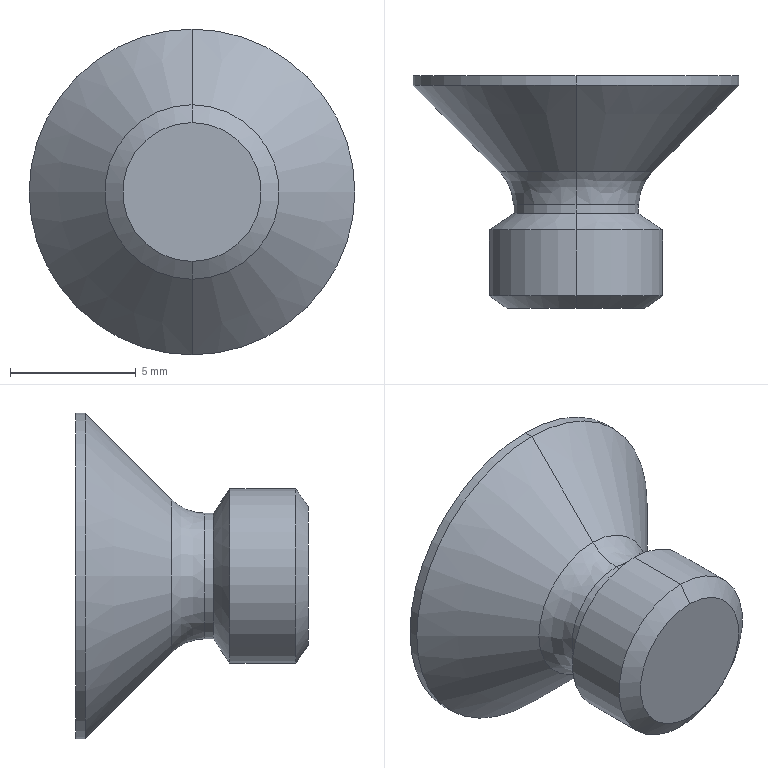Part | SolidWorks | features BaseBody 1 | 1 solid | 31 faces | box 12.923 x 9.231 x 12.923 mm | volume 413.221 mm3 | plane 17 | cylinder 6 | cone 6 | spline 2 | commonest cylinder face diameters 4.988 x2 6.923 x2 12.923 x2
STEP:
#1=CARTESIAN_POINT('',(-17.753,381.039,168.119));
#2=VERTEX_POINT('',#1);
#3=CARTESIAN_POINT('',(-17.753,381.039,174.188));
#4=VERTEX_POINT('',#3);
#5=CARTESIAN_POINT('',(-17.753,381.039,171.154));
#6=DIRECTION('',(0.,1.,0.));
#7=DIRECTION('',(1.,0.,0.));
#8=AXIS2_PLACEMENT_3D('',#5,#6,#7);
#9=CIRCLE('',#8,3.035);
#10=EDGE_CURVE('',#2,#4,#9,.T.);
#11=ORIENTED_EDGE('',*,*,#10,.F.);
#12=CARTESIAN_POINT('',(-17.753,379.733,168.66));
#13=VERTEX_POINT('',#12);
#14=CARTESIAN_POINT('',(-17.753,379.733,166.814));
#15=DIRECTION('',(1.,0.,0.));
#16=DIRECTION('',(0.,0.,-1.));
#17=AXIS2_PLACEMENT_3D('',#14,#15,#16);
#18=CIRCLE('',#17,1.846);
#19=EDGE_CURVE('',#2,#13,#18,.T.);
#20=ORIENTED_EDGE('',*,*,#19,.T.);
#21=CARTESIAN_POINT('',(-17.753,379.733,173.648));
#22=VERTEX_POINT('',#21);
#23=CARTESIAN_POINT('',(-17.753,379.733,171.154));
#24=DIRECTION('',(0.,-1.,0.));
#25=DIRECTION('',(0.,0.,1.));
#26=AXIS2_PLACEMENT_3D('',#23,#24,#25);
#27=CIRCLE('',#26,2.494);
#28=EDGE_CURVE('',#22,#13,#27,.T.);
#29=ORIENTED_EDGE('',*,*,#28,.F.);
#30=CARTESIAN_POINT('',(-17.753,379.733,175.494));
#31=DIRECTION('',(-1.,0.,0.));
#32=DIRECTION('',(0.,0.,1.));
#33=AXIS2_PLACEMENT_3D('',#30,#31,#32);
#34=CIRCLE('',#33,1.846);
#35=EDGE_CURVE('',#4,#22,#34,.T.);
#36=ORIENTED_EDGE('',*,*,#35,.F.);
#37=EDGE_LOOP('',(#11,#20,#29,#36));
#38=FACE_OUTER_BOUND('',#37,.T.);
#39=CARTESIAN_POINT('',(-17.753,381.039,174.188));
#40=CARTESIAN_POINT('',(-23.823,381.039,174.188));
#41=CARTESIAN_POINT('',(-23.823,381.039,168.119));
#42=CARTESIAN_POINT('',(-17.753,381.039,168.119));
#43=CARTESIAN_POINT('',(-17.753,380.688,173.838));
#44=CARTESIAN_POINT('',(-23.121,380.688,173.838));
#45=CARTESIAN_POINT('',(-23.121,380.688,168.47));
#46=CARTESIAN_POINT('',(-17.753,380.688,168.47));
#47=CARTESIAN_POINT('',(-17.753,380.229,173.648));
#48=CARTESIAN_POINT('',(-22.741,380.229,173.648));
#49=CARTESIAN_POINT('',(-22.741,380.229,168.66));
#50=CARTESIAN_POINT('',(-17.753,380.229,168.66));
#51=CARTESIAN_POINT('',(-17.753,379.733,173.648));
#52=CARTESIAN_POINT('',(-22.741,379.733,173.648));
#53=CARTESIAN_POINT('',(-22.741,379.733,168.66));
#54=CARTESIAN_POINT('',(-17.753,379.733,168.66));
#55=(BOUNDED_SURFACE()B_SPLINE_SURFACE(3,3,((#39,#40,#41,#42),(#43,#44,#45,#46),(#47,#48,#49,#50),(#51,#52,#53,#54)),.UNSPECIFIED.,.F.,.F.,.F.)B_SPLINE_SURFACE_WITH_KNOTS((4,4),(4,4),(0.,1.),(0.,1.),.UNSPECIFIED.)GEOMETRIC_REPRESENTATION_ITEM()RATIONAL_B_SPLINE_SURFACE(((1.,0.3333,0.3333,1.),(0.9493,0.3164,0.3164,0.9493),(0.9493,0.3164,0.3164,0.9493),(1.,0.3333,0.3333,1.)))REPRESENTATION_ITEM('')SURFACE());
#56=ADVANCED_FACE('',(#38),#55,.F.);
#57=CARTESIAN_POINT('',(-17.753,384.465,177.615));
#58=VERTEX_POINT('',#57);
#59=CARTESIAN_POINT('',(-17.753,384.465,164.692));
#60=VERTEX_POINT('',#59);
#61=CARTESIAN_POINT('',(-17.753,384.465,171.154));
#62=DIRECTION('',(0.,1.,0.));
#63=DIRECTION('',(0.,0.,1.));
#64=AXIS2_PLACEMENT_3D('',#61,#62,#63);
#65=CIRCLE('',#64,6.462);
#66=EDGE_CURVE('',#58,#60,#65,.T.);
#67=ORIENTED_EDGE('',*,*,#66,.T.);
#68=CARTESIAN_POINT('',(-17.753,384.846,164.692));
#69=VERTEX_POINT('',#68);
#70=CARTESIAN_POINT('',(-17.753,375.615,164.692));
#71=DIRECTION('',(0.,1.,0.));
#72=VECTOR('',#71,1000.);
#73=LINE('',#70,#72);
#74=EDGE_CURVE('',#60,#69,#73,.T.);
#75=ORIENTED_EDGE('',*,*,#74,.T.);
#76=CARTESIAN_POINT('',(-17.753,384.846,177.615));
#77=VERTEX_POINT('',#76);
#78=CARTESIAN_POINT('',(-17.753,384.846,171.154));
#79=DIRECTION('',(0.,-1.,0.));
#80=DIRECTION('',(0.,0.,1.));
#81=AXIS2_PLACEMENT_3D('',#78,#79,#80);
#82=CIRCLE('',#81,6.462);
#83=EDGE_CURVE('',#69,#77,#82,.T.);
#84=ORIENTED_EDGE('',*,*,#83,.T.);
#85=CARTESIAN_POINT('',(-17.753,375.615,177.615));
#86=DIRECTION('',(0.,1.,0.));
#87=VECTOR('',#86,1000.);
#88=LINE('',#85,#87);
#89=EDGE_CURVE('',#58,#77,#88,.T.);
#90=ORIENTED_EDGE('',*,*,#89,.F.);
#91=EDGE_LOOP('',(#67,#75,#84,#90));
#92=FACE_OUTER_BOUND('',#91,.T.);
#93=CARTESIAN_POINT('',(-17.753,375.615,171.154));
#94=DIRECTION('',(0.,1.,0.));
#95=DIRECTION('',(0.,0.,1.));
#96=AXIS2_PLACEMENT_3D('',#93,#94,#95);
#97=CYLINDRICAL_SURFACE('',#96,6.462);
#98=ADVANCED_FACE('',(#92),#97,.T.);
#99=CARTESIAN_POINT('',(-17.753,381.039,171.154));
#100=DIRECTION('',(0.,1.,0.));
#101=DIRECTION('',(1.,0.,0.));
#102=AXIS2_PLACEMENT_3D('',#99,#100,#101);
#103=CIRCLE('',#102,3.035);
#104=EDGE_CURVE('',#4,#2,#103,.T.);
#105=ORIENTED_EDGE('',*,*,#104,.T.);
#106=CARTESIAN_POINT('',(-17.753,384.465,164.692));
#107=DIRECTION('',(0.,0.7071,-0.7071));
#108=VECTOR('',#107,1000.);
#109=LINE('',#106,#108);
#110=EDGE_CURVE('',#2,#60,#109,.T.);
#111=ORIENTED_EDGE('',*,*,#110,.T.);
#112=ORIENTED_EDGE('',*,*,#66,.F.);
#113=CARTESIAN_POINT('',(-17.753,384.465,177.615));
#114=DIRECTION('',(0.,0.7071,0.7071));
#115=VECTOR('',#114,1000.);
#116=LINE('',#113,#115);
#117=EDGE_CURVE('',#4,#58,#116,.T.);
#118=ORIENTED_EDGE('',*,*,#117,.F.);
#119=EDGE_LOOP('',(#105,#111,#112,#118));
#120=FACE_OUTER_BOUND('',#119,.T.);
#121=CARTESIAN_POINT('',(-17.753,384.465,171.154));
#122=DIRECTION('',(0.,1.,0.));
#123=DIRECTION('',(0.,0.,1.));
#124=AXIS2_PLACEMENT_3D('',#121,#122,#123);
#125=CONICAL_SURFACE('',#124,6.462,0.7854);
#126=ADVANCED_FACE('',(#120),#125,.T.);
#127=CARTESIAN_POINT('',(-17.753,379.38,173.648));
#128=VERTEX_POINT('',#127);
#129=CARTESIAN_POINT('',(-17.753,379.38,168.66));
#130=VERTEX_POINT('',#129);
#131=CARTESIAN_POINT('',(-17.753,379.38,171.154));
#132=DIRECTION('',(0.,1.,0.));
#133=DIRECTION('',(0.,0.,1.));
#134=AXIS2_PLACEMENT_3D('',#131,#132,#133);
#135=CIRCLE('',#134,2.494);
#136=EDGE_CURVE('',#128,#130,#135,.T.);
#137=ORIENTED_EDGE('',*,*,#136,.T.);
#138=CARTESIAN_POINT('',(-17.753,375.615,168.66));
#139=DIRECTION('',(0.,1.,0.));
#140=VECTOR('',#139,1000.);
#141=LINE('',#138,#140);
#142=EDGE_CURVE('',#130,#13,#141,.T.);
#143=ORIENTED_EDGE('',*,*,#142,.T.);
#144=CARTESIAN_POINT('',(-17.753,379.733,171.154));
#145=DIRECTION('',(0.,-1.,0.));
#146=DIRECTION('',(0.,0.,1.));
#147=AXIS2_PLACEMENT_3D('',#144,#145,#146);
#148=CIRCLE('',#147,2.494);
#149=EDGE_CURVE('',#13,#22,#148,.T.);
#150=ORIENTED_EDGE('',*,*,#149,.T.);
#151=CARTESIAN_POINT('',(-17.753,375.615,173.648));
#152=DIRECTION('',(0.,1.,0.));
#153=VECTOR('',#152,1000.);
#154=LINE('',#151,#153);
#155=EDGE_CURVE('',#128,#22,#154,.T.);
#156=ORIENTED_EDGE('',*,*,#155,.F.);
#157=EDGE_LOOP('',(#137,#143,#150,#156));
#158=FACE_OUTER_BOUND('',#157,.T.);
#159=CARTESIAN_POINT('',(-17.753,375.615,171.154));
#160=DIRECTION('',(0.,1.,0.));
#161=DIRECTION('',(0.,0.,1.));
#162=AXIS2_PLACEMENT_3D('',#159,#160,#161);
#163=CYLINDRICAL_SURFACE('',#162,2.494);
#164=ADVANCED_FACE('',(#158),#163,.T.);
#165=ORIENTED_EDGE('',*,*,#136,.F.);
#166=CARTESIAN_POINT('',(-17.753,378.731,174.615));
#167=VERTEX_POINT('',#166);
#168=CARTESIAN_POINT('',(-17.753,378.731,174.615));
#169=DIRECTION('',(0.,-0.5573,0.8303));
#170=VECTOR('',#169,1000.);
#171=LINE('',#168,#170);
#172=EDGE_CURVE('',#128,#167,#171,.T.);
#173=ORIENTED_EDGE('',*,*,#172,.T.);
#174=CARTESIAN_POINT('',(-17.753,378.731,167.692));
#175=VERTEX_POINT('',#174);
#176=CARTESIAN_POINT('',(-17.753,378.731,171.154));
#177=DIRECTION('',(0.,1.,0.));
#178=DIRECTION('',(0.,0.,-1.));
#179=AXIS2_PLACEMENT_3D('',#176,#177,#178);
#180=CIRCLE('',#179,3.462);
#181=EDGE_CURVE('',#167,#175,#180,.T.);
#182=ORIENTED_EDGE('',*,*,#181,.T.);
#183=CARTESIAN_POINT('',(-17.753,378.731,167.692));
#184=DIRECTION('',(0.,-0.5573,-0.8303));
#185=VECTOR('',#184,1000.);
#186=LINE('',#183,#185);
#187=EDGE_CURVE('',#130,#175,#186,.T.);
#188=ORIENTED_EDGE('',*,*,#187,.F.);
#189=EDGE_LOOP('',(#165,#173,#182,#188));
#190=FACE_OUTER_BOUND('',#189,.T.);
#191=CARTESIAN_POINT('',(-17.753,378.731,171.154));
#192=DIRECTION('',(0.,-1.,0.));
#193=DIRECTION('',(0.,0.,-1.));
#194=AXIS2_PLACEMENT_3D('',#191,#192,#193);
#195=CONICAL_SURFACE('',#194,3.462,0.9796);
#196=ADVANCED_FACE('',(#190),#195,.T.);
#197=CARTESIAN_POINT('',(-17.753,376.116,174.615));
#198=VERTEX_POINT('',#197);
#199=CARTESIAN_POINT('',(-17.753,376.116,167.692));
#200=VERTEX_POINT('',#199);
#201=CARTESIAN_POINT('',(-17.753,376.116,171.154));
#202=DIRECTION('',(0.,1.,0.));
#203=DIRECTION('',(0.,0.,1.));
#204=AXIS2_PLACEMENT_3D('',#201,#202,#203);
#205=CIRCLE('',#204,3.462);
#206=EDGE_CURVE('',#198,#200,#205,.T.);
#207=ORIENTED_EDGE('',*,*,#206,.T.);
#208=CARTESIAN_POINT('',(-17.753,375.615,167.692));
#209=DIRECTION('',(0.,1.,0.));
#210=VECTOR('',#209,1000.);
#211=LINE('',#208,#210);
#212=EDGE_CURVE('',#200,#175,#211,.T.);
#213=ORIENTED_EDGE('',*,*,#212,.T.);
#214=ORIENTED_EDGE('',*,*,#181,.F.);
#215=CARTESIAN_POINT('',(-17.753,375.615,174.615));
#216=DIRECTION('',(0.,1.,0.));
#217=VECTOR('',#216,1000.);
#218=LINE('',#215,#217);
#219=EDGE_CURVE('',#198,#167,#218,.T.);
#220=ORIENTED_EDGE('',*,*,#219,.F.);
#221=EDGE_LOOP('',(#207,#213,#214,#220));
#222=FACE_OUTER_BOUND('',#221,.T.);
#223=CARTESIAN_POINT('',(-17.753,375.615,171.154));
#224=DIRECTION('',(0.,1.,0.));
#225=DIRECTION('',(0.,0.,1.));
#226=AXIS2_PLACEMENT_3D('',#223,#224,#225);
#227=CYLINDRICAL_SURFACE('',#226,3.462);
#228=ADVANCED_FACE('',(#222),#227,.T.);
#229=CARTESIAN_POINT('',(-17.753,375.615,173.908));
#230=VERTEX_POINT('',#229);
#231=CARTESIAN_POINT('',(-17.753,375.615,168.4));
#232=VERTEX_POINT('',#231);
#233=CARTESIAN_POINT('',(-17.753,375.615,171.154));
#234=DIRECTION('',(0.,1.,0.));
#235=DIRECTION('',(0.,0.,1.));
#236=AXIS2_PLACEMENT_3D('',#233,#234,#235);
#237=CIRCLE('',#236,2.754);
#238=EDGE_CURVE('',#230,#232,#237,.T.);
#239=ORIENTED_EDGE('',*,*,#238,.T.);
#240=CARTESIAN_POINT('',(-17.753,376.116,167.692));
#241=DIRECTION('',(0.,0.5774,-0.8165));
#242=VECTOR('',#241,1000.);
#243=LINE('',#240,#242);
#244=EDGE_CURVE('',#232,#200,#243,.T.);
#245=ORIENTED_EDGE('',*,*,#244,.T.);
#246=ORIENTED_EDGE('',*,*,#206,.F.);
#247=CARTESIAN_POINT('',(-17.753,376.116,174.615));
#248=DIRECTION('',(0.,0.5774,0.8165));
#249=VECTOR('',#248,1000.);
#250=LINE('',#247,#249);
#251=EDGE_CURVE('',#230,#198,#250,.T.);
#252=ORIENTED_EDGE('',*,*,#251,.F.);
#253=EDGE_LOOP('',(#239,#245,#246,#252));
#254=FACE_OUTER_BOUND('',#253,.T.);
#255=CARTESIAN_POINT('',(-17.753,376.116,171.154));
#256=DIRECTION('',(0.,1.,0.));
#257=DIRECTION('',(0.,0.,1.));
#258=AXIS2_PLACEMENT_3D('',#255,#256,#257);
#259=CONICAL_SURFACE('',#258,3.462,0.9553);
#260=ADVANCED_FACE('',(#254),#259,.T.);
#261=CARTESIAN_POINT('',(-21.1,384.846,170.317));
#262=VERTEX_POINT('',#261);
#263=CARTESIAN_POINT('',(-21.1,384.846,171.99));
#264=VERTEX_POINT('',#263);
#265=CARTESIAN_POINT('',(-21.1,384.846,171.154));
#266=DIRECTION('',(0.,0.,1.));
#267=VECTOR('',#266,1000.);
#268=LINE('',#265,#267);
#269=EDGE_CURVE('',#262,#264,#268,.T.);
#270=ORIENTED_EDGE('',*,*,#269,.F.);
#271=CARTESIAN_POINT('',(-18.59,384.846,170.317));
#272=VERTEX_POINT('',#271);
#273=CARTESIAN_POINT('',(-17.753,384.846,170.317));
#274=DIRECTION('',(-1.,0.,0.));
#275=VECTOR('',#274,1000.);
#276=LINE('',#273,#275);
#277=EDGE_CURVE('',#272,#262,#276,.T.);
#278=ORIENTED_EDGE('',*,*,#277,.F.);
#279=CARTESIAN_POINT('',(-18.59,384.846,167.808));
#280=VERTEX_POINT('',#279);
#281=CARTESIAN_POINT('',(-18.59,384.846,171.154));
#282=DIRECTION('',(0.,0.,1.));
#283=VECTOR('',#282,1000.);
#284=LINE('',#281,#283);
#285=EDGE_CURVE('',#280,#272,#284,.T.);
#286=ORIENTED_EDGE('',*,*,#285,.F.);
#287=CARTESIAN_POINT('',(-16.917,384.846,167.808));
#288=VERTEX_POINT('',#287);
#289=CARTESIAN_POINT('',(-17.753,384.846,167.808));
#290=DIRECTION('',(-1.,0.,0.));
#291=VECTOR('',#290,1000.);
#292=LINE('',#289,#291);
#293=EDGE_CURVE('',#288,#280,#292,.T.);
#294=ORIENTED_EDGE('',*,*,#293,.F.);
#295=CARTESIAN_POINT('',(-16.917,384.846,170.317));
#296=VERTEX_POINT('',#295);
#297=CARTESIAN_POINT('',(-16.917,384.846,171.154));
#298=DIRECTION('',(0.,0.,-1.));
#299=VECTOR('',#298,1000.);
#300=LINE('',#297,#299);
#301=EDGE_CURVE('',#296,#288,#300,.T.);
#302=ORIENTED_EDGE('',*,*,#301,.F.);
#303=CARTESIAN_POINT('',(-14.407,384.846,170.317));
#304=VERTEX_POINT('',#303);
#305=CARTESIAN_POINT('',(-17.753,384.846,170.317));
#306=DIRECTION('',(-1.,0.,0.));
#307=VECTOR('',#306,1000.);
#308=LINE('',#305,#307);
#309=EDGE_CURVE('',#304,#296,#308,.T.);
#310=ORIENTED_EDGE('',*,*,#309,.F.);
#311=CARTESIAN_POINT('',(-14.407,384.846,171.99));
#312=VERTEX_POINT('',#311);
#313=CARTESIAN_POINT('',(-14.407,384.846,171.154));
#314=DIRECTION('',(0.,0.,-1.));
#315=VECTOR('',#314,1000.);
#316=LINE('',#313,#315);
#317=EDGE_CURVE('',#312,#304,#316,.T.);
#318=ORIENTED_EDGE('',*,*,#317,.F.);
#319=CARTESIAN_POINT('',(-16.917,384.846,171.99));
#320=VERTEX_POINT('',#319);
#321=CARTESIAN_POINT('',(-17.753,384.846,171.99));
#322=DIRECTION('',(1.,0.,0.));
#323=VECTOR('',#322,1000.);
#324=LINE('',#321,#323);
#325=EDGE_CURVE('',#320,#312,#324,.T.);
#326=ORIENTED_EDGE('',*,*,#325,.F.);
#327=CARTESIAN_POINT('',(-16.917,384.846,174.5));
#328=VERTEX_POINT('',#327);
#329=CARTESIAN_POINT('',(-16.917,384.846,171.154));
#330=DIRECTION('',(0.,0.,-1.));
#331=VECTOR('',#330,1000.);
#332=LINE('',#329,#331);
#333=EDGE_CURVE('',#328,#320,#332,.T.);
#334=ORIENTED_EDGE('',*,*,#333,.F.);
#335=CARTESIAN_POINT('',(-18.59,384.846,174.5));
#336=VERTEX_POINT('',#335);
#337=CARTESIAN_POINT('',(-17.753,384.846,174.5));
#338=DIRECTION('',(1.,0.,0.));
#339=VECTOR('',#338,1000.);
#340=LINE('',#337,#339);
#341=EDGE_CURVE('',#336,#328,#340,.T.);
#342=ORIENTED_EDGE('',*,*,#341,.F.);
#343=CARTESIAN_POINT('',(-18.59,384.846,171.99));
#344=VERTEX_POINT('',#343);
#345=CARTESIAN_POINT('',(-18.59,384.846,171.154));
#346=DIRECTION('',(0.,0.,1.));
#347=VECTOR('',#346,1000.);
#348=LINE('',#345,#347);
#349=EDGE_CURVE('',#344,#336,#348,.T.);
#350=ORIENTED_EDGE('',*,*,#349,.F.);
#351=CARTESIAN_POINT('',(-17.753,384.846,171.99));
#352=DIRECTION('',(1.,0.,0.));
#353=VECTOR('',#352,1000.);
#354=LINE('',#351,#353);
#355=EDGE_CURVE('',#264,#344,#354,.T.);
#356=ORIENTED_EDGE('',*,*,#355,.F.);
#357=EDGE_LOOP('',(#270,#278,#286,#294,#302,#310,#318,#326,#334,#342,#350,#356));
#358=FACE_BOUND('',#357,.T.);
#359=CARTESIAN_POINT('',(-17.753,384.846,171.154));
#360=DIRECTION('',(0.,-1.,0.));
#361=DIRECTION('',(0.,0.,1.));
#362=AXIS2_PLACEMENT_3D('',#359,#360,#361);
#363=CIRCLE('',#362,6.462);
#364=EDGE_CURVE('',#77,#69,#363,.T.);
#365=ORIENTED_EDGE('',*,*,#364,.F.);
#366=ORIENTED_EDGE('',*,*,#83,.F.);
#367=EDGE_LOOP('',(#365,#366));
#368=FACE_OUTER_BOUND('',#367,.T.);
#369=CARTESIAN_POINT('',(-17.753,384.846,171.154));
#370=DIRECTION('',(0.,-1.,0.));
#371=DIRECTION('',(0.,0.,-1.));
#372=AXIS2_PLACEMENT_3D('',#369,#370,#371);
#373=PLANE('',#372);
#374=ADVANCED_FACE('',(#358,#368),#373,.F.);
#375=CARTESIAN_POINT('',(-21.1,382.942,171.99));
#376=VERTEX_POINT('',#375);
#377=CARTESIAN_POINT('',(-21.1,384.846,171.99));
#378=DIRECTION('',(0.,-1.,0.));
#379=VECTOR('',#378,1000.);
#380=LINE('',#377,#379);
#381=EDGE_CURVE('',#264,#376,#380,.T.);
#382=ORIENTED_EDGE('',*,*,#381,.F.);
#383=ORIENTED_EDGE('',*,*,#355,.T.);
#384=CARTESIAN_POINT('',(-18.59,381.241,171.99));
#385=VERTEX_POINT('',#384);
#386=CARTESIAN_POINT('',(-18.59,384.846,171.99));
#387=DIRECTION('',(0.,1.,0.));
#388=VECTOR('',#387,1000.);
#389=LINE('',#386,#388);
#390=EDGE_CURVE('',#385,#344,#389,.T.);
#391=ORIENTED_EDGE('',*,*,#390,.F.);
#392=CARTESIAN_POINT('',(-21.1,382.942,171.99));
#393=DIRECTION('',(0.8278,-0.5611,0.));
#394=VECTOR('',#393,1000.);
#395=LINE('',#392,#394);
#396=EDGE_CURVE('',#376,#385,#395,.T.);
#397=ORIENTED_EDGE('',*,*,#396,.F.);
#398=EDGE_LOOP('',(#382,#383,#391,#397));
#399=FACE_OUTER_BOUND('',#398,.T.);
#400=CARTESIAN_POINT('',(-17.753,384.846,171.99));
#401=DIRECTION('',(0.,0.,1.));
#402=DIRECTION('',(1.,0.,0.));
#403=AXIS2_PLACEMENT_3D('',#400,#401,#402);
#404=PLANE('',#403);
#405=ADVANCED_FACE('',(#399),#404,.F.);
#406=ORIENTED_EDGE('',*,*,#381,.T.);
#407=CARTESIAN_POINT('',(-21.1,382.942,170.317));
#408=VERTEX_POINT('',#407);
#409=CARTESIAN_POINT('',(-21.1,382.942,171.99));
#410=DIRECTION('',(0.,0.,-1.));
#411=VECTOR('',#410,1000.);
#412=LINE('',#409,#411);
#413=EDGE_CURVE('',#376,#408,#412,.T.);
#414=ORIENTED_EDGE('',*,*,#413,.T.);
#415=CARTESIAN_POINT('',(-21.1,394.458,170.317));
#416=DIRECTION('',(0.,1.,0.));
#417=VECTOR('',#416,1000.);
#418=LINE('',#415,#417);
#419=EDGE_CURVE('',#408,#262,#418,.T.);
#420=ORIENTED_EDGE('',*,*,#419,.T.);
#421=ORIENTED_EDGE('',*,*,#269,.T.);
#422=EDGE_LOOP('',(#406,#414,#420,#421));
#423=FACE_OUTER_BOUND('',#422,.T.);
#424=CARTESIAN_POINT('',(-21.1,394.458,171.99));
#425=DIRECTION('',(1.,0.,0.));
#426=DIRECTION('',(0.,0.,-1.));
#427=AXIS2_PLACEMENT_3D('',#424,#425,#426);
#428=PLANE('',#427);
#429=ADVANCED_FACE('',(#423),#428,.T.);
#430=ORIENTED_EDGE('',*,*,#277,.T.);
#431=ORIENTED_EDGE('',*,*,#419,.F.);
#432=CARTESIAN_POINT('',(-18.59,381.241,170.317));
#433=VERTEX_POINT('',#432);
#434=CARTESIAN_POINT('',(-21.1,382.942,170.317));
#435=DIRECTION('',(0.8278,-0.5611,0.));
#436=VECTOR('',#435,1000.);
#437=LINE('',#434,#436);
#438=EDGE_CURVE('',#408,#433,#437,.T.);
#439=ORIENTED_EDGE('',*,*,#438,.T.);
#440=CARTESIAN_POINT('',(-18.59,384.846,170.317));
#441=DIRECTION('',(0.,1.,0.));
#442=VECTOR('',#441,1000.);
#443=LINE('',#440,#442);
#444=EDGE_CURVE('',#433,#272,#443,.T.);
#445=ORIENTED_EDGE('',*,*,#444,.T.);
#446=EDGE_LOOP('',(#430,#431,#439,#445));
#447=FACE_OUTER_BOUND('',#446,.T.);
#448=CARTESIAN_POINT('',(-17.753,384.846,170.317));
#449=DIRECTION('',(0.,0.,1.));
#450=DIRECTION('',(1.,0.,0.));
#451=AXIS2_PLACEMENT_3D('',#448,#449,#450);
#452=PLANE('',#451);
#453=ADVANCED_FACE('',(#447),#452,.T.);
#454=CARTESIAN_POINT('',(-18.59,382.942,167.808));
#455=VERTEX_POINT('',#454);
#456=CARTESIAN_POINT('',(-18.59,381.01,170.317));
#457=VERTEX_POINT('',#456);
#458=CARTESIAN_POINT('',(-18.59,382.942,167.808));
#459=DIRECTION('',(0.,-0.61,0.7924));
#460=VECTOR('',#459,1000.);
#461=LINE('',#458,#460);
#462=EDGE_CURVE('',#455,#457,#461,.T.);
#463=ORIENTED_EDGE('',*,*,#462,.F.);
#464=CARTESIAN_POINT('',(-18.59,384.846,167.808));
#465=DIRECTION('',(0.,-1.,0.));
#466=VECTOR('',#465,1000.);
#467=LINE('',#464,#466);
#468=EDGE_CURVE('',#280,#455,#467,.T.);
#469=ORIENTED_EDGE('',*,*,#468,.F.);
#470=ORIENTED_EDGE('',*,*,#285,.T.);
#471=ORIENTED_EDGE('',*,*,#444,.F.);
#472=CARTESIAN_POINT('',(-18.59,381.241,171.154));
#473=DIRECTION('',(0.,0.,-1.));
#474=VECTOR('',#473,1000.);
#475=LINE('',#472,#474);
#476=EDGE_CURVE('',#385,#433,#475,.T.);
#477=ORIENTED_EDGE('',*,*,#476,.F.);
#478=ORIENTED_EDGE('',*,*,#390,.T.);
#479=ORIENTED_EDGE('',*,*,#349,.T.);
#480=CARTESIAN_POINT('',(-18.59,382.942,174.5));
#481=VERTEX_POINT('',#480);
#482=CARTESIAN_POINT('',(-18.59,384.846,174.5));
#483=DIRECTION('',(0.,1.,0.));
#484=VECTOR('',#483,1000.);
#485=LINE('',#482,#484);
#486=EDGE_CURVE('',#481,#336,#485,.T.);
#487=ORIENTED_EDGE('',*,*,#486,.F.);
#488=CARTESIAN_POINT('',(-18.59,381.01,171.99));
#489=VERTEX_POINT('',#488);
#490=CARTESIAN_POINT('',(-18.59,381.01,171.99));
#491=DIRECTION('',(0.,0.61,0.7924));
#492=VECTOR('',#491,1000.);
#493=LINE('',#490,#492);
#494=EDGE_CURVE('',#489,#481,#493,.T.);
#495=ORIENTED_EDGE('',*,*,#494,.F.);
#496=CARTESIAN_POINT('',(-18.59,381.01,171.154));
#497=DIRECTION('',(0.,0.,1.));
#498=VECTOR('',#497,1000.);
#499=LINE('',#496,#498);
#500=EDGE_CURVE('',#457,#489,#499,.T.);
#501=ORIENTED_EDGE('',*,*,#500,.F.);
#502=EDGE_LOOP('',(#463,#469,#470,#471,#477,#478,#479,#487,#495,#501));
#503=FACE_OUTER_BOUND('',#502,.T.);
#504=CARTESIAN_POINT('',(-18.59,384.846,171.154));
#505=DIRECTION('',(-1.,0.,0.));
#506=DIRECTION('',(0.,0.,1.));
#507=AXIS2_PLACEMENT_3D('',#504,#505,#506);
#508=PLANE('',#507);
#509=ADVANCED_FACE('',(#503),#508,.F.);
#510=ORIENTED_EDGE('',*,*,#468,.T.);
#511=CARTESIAN_POINT('',(-16.917,382.942,167.808));
#512=VERTEX_POINT('',#511);
#513=CARTESIAN_POINT('',(-18.59,382.942,167.808));
#514=DIRECTION('',(1.,0.,0.));
#515=VECTOR('',#514,1000.);
#516=LINE('',#513,#515);
#517=EDGE_CURVE('',#455,#512,#516,.T.);
#518=ORIENTED_EDGE('',*,*,#517,.T.);
#519=CARTESIAN_POINT('',(-16.917,385.227,167.808));
#520=DIRECTION('',(0.,1.,0.));
#521=VECTOR('',#520,1000.);
#522=LINE('',#519,#521);
#523=EDGE_CURVE('',#512,#288,#522,.T.);
#524=ORIENTED_EDGE('',*,*,#523,.T.);
#525=ORIENTED_EDGE('',*,*,#293,.T.);
#526=EDGE_LOOP('',(#510,#518,#524,#525));
#527=FACE_OUTER_BOUND('',#526,.T.);
#528=CARTESIAN_POINT('',(-18.59,385.227,167.808));
#529=DIRECTION('',(0.,0.,1.));
#530=DIRECTION('',(1.,0.,0.));
#531=AXIS2_PLACEMENT_3D('',#528,#529,#530);
#532=PLANE('',#531);
#533=ADVANCED_FACE('',(#527),#532,.T.);
#534=CARTESIAN_POINT('',(-16.917,381.01,170.317));
#535=VERTEX_POINT('',#534);
#536=CARTESIAN_POINT('',(-16.917,381.01,171.99));
#537=VERTEX_POINT('',#536);
#538=CARTESIAN_POINT('',(-16.917,381.01,171.154));
#539=DIRECTION('',(0.,0.,1.));
#540=VECTOR('',#539,1000.);
#541=LINE('',#538,#540);
#542=EDGE_CURVE('',#535,#537,#541,.T.);
#543=ORIENTED_EDGE('',*,*,#542,.T.);
#544=CARTESIAN_POINT('',(-16.917,382.942,174.5));
#545=VERTEX_POINT('',#544);
#546=CARTESIAN_POINT('',(-16.917,381.01,171.99));
#547=DIRECTION('',(0.,0.61,0.7924));
#548=VECTOR('',#547,1000.);
#549=LINE('',#546,#548);
#550=EDGE_CURVE('',#537,#545,#549,.T.);
#551=ORIENTED_EDGE('',*,*,#550,.T.);
#552=CARTESIAN_POINT('',(-16.917,384.846,174.5));
#553=DIRECTION('',(0.,1.,0.));
#554=VECTOR('',#553,1000.);
#555=LINE('',#552,#554);
#556=EDGE_CURVE('',#545,#328,#555,.T.);
#557=ORIENTED_EDGE('',*,*,#556,.T.);
#558=ORIENTED_EDGE('',*,*,#333,.T.);
#559=CARTESIAN_POINT('',(-16.917,381.241,171.99));
#560=VERTEX_POINT('',#559);
#561=CARTESIAN_POINT('',(-16.917,384.846,171.99));
#562=DIRECTION('',(0.,-1.,0.));
#563=VECTOR('',#562,1000.);
#564=LINE('',#561,#563);
#565=EDGE_CURVE('',#320,#560,#564,.T.);
#566=ORIENTED_EDGE('',*,*,#565,.T.);
#567=CARTESIAN_POINT('',(-16.917,381.241,170.317));
#568=VERTEX_POINT('',#567);
#569=CARTESIAN_POINT('',(-16.917,381.241,171.154));
#570=DIRECTION('',(0.,0.,-1.));
#571=VECTOR('',#570,1000.);
#572=LINE('',#569,#571);
#573=EDGE_CURVE('',#560,#568,#572,.T.);
#574=ORIENTED_EDGE('',*,*,#573,.T.);
#575=CARTESIAN_POINT('',(-16.917,384.846,170.317));
#576=DIRECTION('',(0.,1.,0.));
#577=VECTOR('',#576,1000.);
#578=LINE('',#575,#577);
#579=EDGE_CURVE('',#568,#296,#578,.T.);
#580=ORIENTED_EDGE('',*,*,#579,.T.);
#581=ORIENTED_EDGE('',*,*,#301,.T.);
#582=ORIENTED_EDGE('',*,*,#523,.F.);
#583=CARTESIAN_POINT('',(-16.917,382.942,167.808));
#584=DIRECTION('',(0.,-0.61,0.7924));
#585=VECTOR('',#584,1000.);
#586=LINE('',#583,#585);
#587=EDGE_CURVE('',#512,#535,#586,.T.);
#588=ORIENTED_EDGE('',*,*,#587,.T.);
#589=EDGE_LOOP('',(#543,#551,#557,#558,#566,#574,#580,#581,#582,#588));
#590=FACE_OUTER_BOUND('',#589,.T.);
#591=CARTESIAN_POINT('',(-16.917,384.846,171.154));
#592=DIRECTION('',(-1.,0.,0.));
#593=DIRECTION('',(0.,0.,1.));
#594=AXIS2_PLACEMENT_3D('',#591,#592,#593);
#595=PLANE('',#594);
#596=ADVANCED_FACE('',(#590),#595,.T.);
#597=ORIENTED_EDGE('',*,*,#579,.F.);
#598=CARTESIAN_POINT('',(-14.407,382.942,170.317));
#599=VERTEX_POINT('',#598);
#600=CARTESIAN_POINT('',(-16.917,381.241,170.317));
#601=DIRECTION('',(0.8278,0.5611,0.));
#602=VECTOR('',#601,1000.);
#603=LINE('',#600,#602);
#604=EDGE_CURVE('',#568,#599,#603,.T.);
#605=ORIENTED_EDGE('',*,*,#604,.T.);
#606=CARTESIAN_POINT('',(-14.407,384.846,170.317));
#607=DIRECTION('',(0.,1.,0.));
#608=VECTOR('',#607,1000.);
#609=LINE('',#606,#608);
#610=EDGE_CURVE('',#599,#304,#609,.T.);
#611=ORIENTED_EDGE('',*,*,#610,.T.);
#612=ORIENTED_EDGE('',*,*,#309,.T.);
#613=EDGE_LOOP('',(#597,#605,#611,#612));
#614=FACE_OUTER_BOUND('',#613,.T.);
#615=CARTESIAN_POINT('',(-17.753,384.846,170.317));
#616=DIRECTION('',(0.,0.,1.));
#617=DIRECTION('',(1.,0.,0.));
#618=AXIS2_PLACEMENT_3D('',#615,#616,#617);
#619=PLANE('',#618);
#620=ADVANCED_FACE('',(#614),#619,.T.);
#621=ORIENTED_EDGE('',*,*,#317,.T.);
#622=ORIENTED_EDGE('',*,*,#610,.F.);
#623=CARTESIAN_POINT('',(-14.407,382.942,171.99));
#624=VERTEX_POINT('',#623);
#625=CARTESIAN_POINT('',(-14.407,382.942,171.99));
#626=DIRECTION('',(0.,0.,1.));
#627=VECTOR('',#626,1000.);
#628=LINE('',#625,#627);
#629=EDGE_CURVE('',#599,#624,#628,.T.);
#630=ORIENTED_EDGE('',*,*,#629,.T.);
#631=CARTESIAN_POINT('',(-14.407,382.942,171.99));
#632=DIRECTION('',(0.,1.,0.));
#633=VECTOR('',#632,1000.);
#634=LINE('',#631,#633);
#635=EDGE_CURVE('',#624,#312,#634,.T.);
#636=ORIENTED_EDGE('',*,*,#635,.T.);
#637=EDGE_LOOP('',(#621,#622,#630,#636));
#638=FACE_OUTER_BOUND('',#637,.T.);
#639=CARTESIAN_POINT('',(-14.407,382.942,171.99));
#640=DIRECTION('',(-1.,0.,0.));
#641=DIRECTION('',(0.,0.,1.));
#642=AXIS2_PLACEMENT_3D('',#639,#640,#641);
#643=PLANE('',#642);
#644=ADVANCED_FACE('',(#638),#643,.T.);
#645=CARTESIAN_POINT('',(-16.917,381.241,171.99));
#646=DIRECTION('',(0.8278,0.5611,0.));
#647=VECTOR('',#646,1000.);
#648=LINE('',#645,#647);
#649=EDGE_CURVE('',#560,#624,#648,.T.);
#650=ORIENTED_EDGE('',*,*,#649,.F.);
#651=ORIENTED_EDGE('',*,*,#565,.F.);
#652=ORIENTED_EDGE('',*,*,#325,.T.);
#653=ORIENTED_EDGE('',*,*,#635,.F.);
#654=EDGE_LOOP('',(#650,#651,#652,#653));
#655=FACE_OUTER_BOUND('',#654,.T.);
#656=CARTESIAN_POINT('',(-17.753,384.846,171.99));
#657=DIRECTION('',(0.,0.,1.));
#658=DIRECTION('',(1.,0.,0.));
#659=AXIS2_PLACEMENT_3D('',#656,#657,#658);
#660=PLANE('',#659);
#661=ADVANCED_FACE('',(#655),#660,.F.);
#662=ORIENTED_EDGE('',*,*,#556,.F.);
#663=CARTESIAN_POINT('',(-18.59,382.942,174.5));
#664=DIRECTION('',(-1.,0.,0.));
#665=VECTOR('',#664,1000.);
#666=LINE('',#663,#665);
#667=EDGE_CURVE('',#545,#481,#666,.T.);
#668=ORIENTED_EDGE('',*,*,#667,.T.);
#669=ORIENTED_EDGE('',*,*,#486,.T.);
#670=ORIENTED_EDGE('',*,*,#341,.T.);
#671=EDGE_LOOP('',(#662,#668,#669,#670));
#672=FACE_OUTER_BOUND('',#671,.T.);
#673=CARTESIAN_POINT('',(-18.59,382.942,174.5));
#674=DIRECTION('',(0.,0.,-1.));
#675=DIRECTION('',(-1.,0.,0.));
#676=AXIS2_PLACEMENT_3D('',#673,#674,#675);
#677=PLANE('',#676);
#678=ADVANCED_FACE('',(#672),#677,.T.);
#679=ORIENTED_EDGE('',*,*,#74,.F.);
#680=CARTESIAN_POINT('',(-17.753,384.465,171.154));
#681=DIRECTION('',(0.,1.,0.));
#682=DIRECTION('',(0.,0.,1.));
#683=AXIS2_PLACEMENT_3D('',#680,#681,#682);
#684=CIRCLE('',#683,6.462);
#685=EDGE_CURVE('',#60,#58,#684,.T.);
#686=ORIENTED_EDGE('',*,*,#685,.T.);
#687=ORIENTED_EDGE('',*,*,#89,.T.);
#688=ORIENTED_EDGE('',*,*,#364,.T.);
#689=EDGE_LOOP('',(#679,#686,#687,#688));
#690=FACE_OUTER_BOUND('',#689,.T.);
#691=CARTESIAN_POINT('',(-17.753,375.615,171.154));
#692=DIRECTION('',(0.,1.,0.));
#693=DIRECTION('',(0.,0.,1.));
#694=AXIS2_PLACEMENT_3D('',#691,#692,#693);
#695=CYLINDRICAL_SURFACE('',#694,6.462);
#696=ADVANCED_FACE('',(#690),#695,.T.);
#697=ORIENTED_EDGE('',*,*,#413,.F.);
#698=ORIENTED_EDGE('',*,*,#396,.T.);
#699=ORIENTED_EDGE('',*,*,#476,.T.);
#700=ORIENTED_EDGE('',*,*,#438,.F.);
#701=EDGE_LOOP('',(#697,#698,#699,#700));
#702=FACE_OUTER_BOUND('',#701,.T.);
#703=CARTESIAN_POINT('',(-21.1,382.942,171.99));
#704=DIRECTION('',(0.5611,0.8278,0.));
#705=DIRECTION('',(-0.8278,0.5611,0.));
#706=AXIS2_PLACEMENT_3D('',#703,#704,#705);
#707=PLANE('',#706);
#708=ADVANCED_FACE('',(#702),#707,.T.);
#709=CARTESIAN_POINT('',(-18.59,381.01,170.317));
#710=DIRECTION('',(-1.,0.,0.));
#711=VECTOR('',#710,1000.);
#712=LINE('',#709,#711);
#713=EDGE_CURVE('',#535,#457,#712,.T.);
#714=ORIENTED_EDGE('',*,*,#713,.T.);
#715=ORIENTED_EDGE('',*,*,#500,.T.);
#716=CARTESIAN_POINT('',(-18.59,381.01,171.99));
#717=DIRECTION('',(1.,0.,0.));
#718=VECTOR('',#717,1000.);
#719=LINE('',#716,#718);
#720=EDGE_CURVE('',#489,#537,#719,.T.);
#721=ORIENTED_EDGE('',*,*,#720,.T.);
#722=ORIENTED_EDGE('',*,*,#542,.F.);
#723=EDGE_LOOP('',(#714,#715,#721,#722));
#724=FACE_OUTER_BOUND('',#723,.T.);
#725=CARTESIAN_POINT('',(-18.59,381.01,170.317));
#726=DIRECTION('',(0.,1.,0.));
#727=DIRECTION('',(0.,0.,1.));
#728=AXIS2_PLACEMENT_3D('',#725,#726,#727);
#729=PLANE('',#728);
#730=ADVANCED_FACE('',(#724),#729,.T.);
#731=ORIENTED_EDGE('',*,*,#517,.F.);
#732=ORIENTED_EDGE('',*,*,#462,.T.);
#733=ORIENTED_EDGE('',*,*,#713,.F.);
#734=ORIENTED_EDGE('',*,*,#587,.F.);
#735=EDGE_LOOP('',(#731,#732,#733,#734));
#736=FACE_OUTER_BOUND('',#735,.T.);
#737=CARTESIAN_POINT('',(-18.59,382.942,167.808));
#738=DIRECTION('',(0.,0.7924,0.61));
#739=DIRECTION('',(0.,-0.61,0.7924));
#740=AXIS2_PLACEMENT_3D('',#737,#738,#739);
#741=PLANE('',#740);
#742=ADVANCED_FACE('',(#736),#741,.T.);
#743=ORIENTED_EDGE('',*,*,#720,.F.);
#744=ORIENTED_EDGE('',*,*,#494,.T.);
#745=ORIENTED_EDGE('',*,*,#667,.F.);
#746=ORIENTED_EDGE('',*,*,#550,.F.);
#747=EDGE_LOOP('',(#743,#744,#745,#746));
#748=FACE_OUTER_BOUND('',#747,.T.);
#749=CARTESIAN_POINT('',(-18.59,381.01,171.99));
#750=DIRECTION('',(0.,0.7924,-0.61));
#751=DIRECTION('',(0.,0.61,0.7924));
#752=AXIS2_PLACEMENT_3D('',#749,#750,#751);
#753=PLANE('',#752);
#754=ADVANCED_FACE('',(#748),#753,.T.);
#755=ORIENTED_EDGE('',*,*,#573,.F.);
#756=ORIENTED_EDGE('',*,*,#649,.T.);
#757=ORIENTED_EDGE('',*,*,#629,.F.);
#758=ORIENTED_EDGE('',*,*,#604,.F.);
#759=EDGE_LOOP('',(#755,#756,#757,#758));
#760=FACE_OUTER_BOUND('',#759,.T.);
#761=CARTESIAN_POINT('',(-16.917,381.241,171.99));
#762=DIRECTION('',(-0.5611,0.8278,0.));
#763=DIRECTION('',(-0.8278,-0.5611,0.));
#764=AXIS2_PLACEMENT_3D('',#761,#762,#763);
#765=PLANE('',#764);
#766=ADVANCED_FACE('',(#760),#765,.T.);
#767=ORIENTED_EDGE('',*,*,#110,.F.);
#768=ORIENTED_EDGE('',*,*,#10,.T.);
#769=ORIENTED_EDGE('',*,*,#117,.T.);
#770=ORIENTED_EDGE('',*,*,#685,.F.);
#771=EDGE_LOOP('',(#767,#768,#769,#770));
#772=FACE_OUTER_BOUND('',#771,.T.);
#773=CARTESIAN_POINT('',(-17.753,384.465,171.154));
#774=DIRECTION('',(0.,1.,0.));
#775=DIRECTION('',(0.,0.,1.));
#776=AXIS2_PLACEMENT_3D('',#773,#774,#775);
#777=CONICAL_SURFACE('',#776,6.462,0.7854);
#778=ADVANCED_FACE('',(#772),#777,.T.);
#779=ORIENTED_EDGE('',*,*,#19,.F.);
#780=ORIENTED_EDGE('',*,*,#104,.F.);
#781=ORIENTED_EDGE('',*,*,#35,.T.);
#782=ORIENTED_EDGE('',*,*,#149,.F.);
#783=EDGE_LOOP('',(#779,#780,#781,#782));
#784=FACE_OUTER_BOUND('',#783,.T.);
#785=CARTESIAN_POINT('',(-17.753,381.039,168.119));
#786=CARTESIAN_POINT('',(-11.684,381.039,168.119));
#787=CARTESIAN_POINT('',(-11.684,381.039,174.188));
#788=CARTESIAN_POINT('',(-17.753,381.039,174.188));
#789=CARTESIAN_POINT('',(-17.753,380.688,168.47));
#790=CARTESIAN_POINT('',(-12.386,380.688,168.47));
#791=CARTESIAN_POINT('',(-12.386,380.688,173.838));
#792=CARTESIAN_POINT('',(-17.753,380.688,173.838));
#793=CARTESIAN_POINT('',(-17.753,380.229,168.66));
#794=CARTESIAN_POINT('',(-12.766,380.229,168.66));
#795=CARTESIAN_POINT('',(-12.766,380.229,173.648));
#796=CARTESIAN_POINT('',(-17.753,380.229,173.648));
#797=CARTESIAN_POINT('',(-17.753,379.733,168.66));
#798=CARTESIAN_POINT('',(-12.766,379.733,168.66));
#799=CARTESIAN_POINT('',(-12.766,379.733,173.648));
#800=CARTESIAN_POINT('',(-17.753,379.733,173.648));
#801=(BOUNDED_SURFACE()B_SPLINE_SURFACE(3,3,((#785,#786,#787,#788),(#789,#790,#791,#792),(#793,#794,#795,#796),(#797,#798,#799,#800)),.UNSPECIFIED.,.F.,.F.,.T.)B_SPLINE_SURFACE_WITH_KNOTS((4,4),(4,4),(0.,1.),(0.,1.),.UNSPECIFIED.)GEOMETRIC_REPRESENTATION_ITEM()RATIONAL_B_SPLINE_SURFACE(((1.,0.3333,0.3333,1.),(0.9493,0.3164,0.3164,0.9493),(0.9493,0.3164,0.3164,0.9493),(1.,0.3333,0.3333,1.)))REPRESENTATION_ITEM('')SURFACE());
#802=ADVANCED_FACE('',(#784),#801,.F.);
#803=ORIENTED_EDGE('',*,*,#142,.F.);
#804=CARTESIAN_POINT('',(-17.753,379.38,171.154));
#805=DIRECTION('',(0.,1.,0.));
#806=DIRECTION('',(0.,0.,1.));
#807=AXIS2_PLACEMENT_3D('',#804,#805,#806);
#808=CIRCLE('',#807,2.494);
#809=EDGE_CURVE('',#130,#128,#808,.T.);
#810=ORIENTED_EDGE('',*,*,#809,.T.);
#811=ORIENTED_EDGE('',*,*,#155,.T.);
#812=ORIENTED_EDGE('',*,*,#28,.T.);
#813=EDGE_LOOP('',(#803,#810,#811,#812));
#814=FACE_OUTER_BOUND('',#813,.T.);
#815=CARTESIAN_POINT('',(-17.753,375.615,171.154));
#816=DIRECTION('',(0.,1.,0.));
#817=DIRECTION('',(0.,0.,1.));
#818=AXIS2_PLACEMENT_3D('',#815,#816,#817);
#819=CYLINDRICAL_SURFACE('',#818,2.494);
#820=ADVANCED_FACE('',(#814),#819,.T.);
#821=ORIENTED_EDGE('',*,*,#172,.F.);
#822=ORIENTED_EDGE('',*,*,#809,.F.);
#823=ORIENTED_EDGE('',*,*,#187,.T.);
#824=CARTESIAN_POINT('',(-17.753,378.731,171.154));
#825=DIRECTION('',(0.,1.,0.));
#826=DIRECTION('',(0.,0.,-1.));
#827=AXIS2_PLACEMENT_3D('',#824,#825,#826);
#828=CIRCLE('',#827,3.462);
#829=EDGE_CURVE('',#175,#167,#828,.T.);
#830=ORIENTED_EDGE('',*,*,#829,.T.);
#831=EDGE_LOOP('',(#821,#822,#823,#830));
#832=FACE_OUTER_BOUND('',#831,.T.);
#833=CARTESIAN_POINT('',(-17.753,378.731,171.154));
#834=DIRECTION('',(0.,-1.,0.));
#835=DIRECTION('',(0.,0.,-1.));
#836=AXIS2_PLACEMENT_3D('',#833,#834,#835);
#837=CONICAL_SURFACE('',#836,3.462,0.9796);
#838=ADVANCED_FACE('',(#832),#837,.T.);
#839=ORIENTED_EDGE('',*,*,#212,.F.);
#840=CARTESIAN_POINT('',(-17.753,376.116,171.154));
#841=DIRECTION('',(0.,1.,0.));
#842=DIRECTION('',(0.,0.,1.));
#843=AXIS2_PLACEMENT_3D('',#840,#841,#842);
#844=CIRCLE('',#843,3.462);
#845=EDGE_CURVE('',#200,#198,#844,.T.);
#846=ORIENTED_EDGE('',*,*,#845,.T.);
#847=ORIENTED_EDGE('',*,*,#219,.T.);
#848=ORIENTED_EDGE('',*,*,#829,.F.);
#849=EDGE_LOOP('',(#839,#846,#847,#848));
#850=FACE_OUTER_BOUND('',#849,.T.);
#851=CARTESIAN_POINT('',(-17.753,375.615,171.154));
#852=DIRECTION('',(0.,1.,0.));
#853=DIRECTION('',(0.,0.,1.));
#854=AXIS2_PLACEMENT_3D('',#851,#852,#853);
#855=CYLINDRICAL_SURFACE('',#854,3.462);
#856=ADVANCED_FACE('',(#850),#855,.T.);
#857=ORIENTED_EDGE('',*,*,#244,.F.);
#858=CARTESIAN_POINT('',(-17.753,375.615,171.154));
#859=DIRECTION('',(0.,1.,0.));
#860=DIRECTION('',(0.,0.,1.));
#861=AXIS2_PLACEMENT_3D('',#858,#859,#860);
#862=CIRCLE('',#861,2.754);
#863=EDGE_CURVE('',#232,#230,#862,.T.);
#864=ORIENTED_EDGE('',*,*,#863,.T.);
#865=ORIENTED_EDGE('',*,*,#251,.T.);
#866=ORIENTED_EDGE('',*,*,#845,.F.);
#867=EDGE_LOOP('',(#857,#864,#865,#866));
#868=FACE_OUTER_BOUND('',#867,.T.);
#869=CARTESIAN_POINT('',(-17.753,376.116,171.154));
#870=DIRECTION('',(0.,1.,0.));
#871=DIRECTION('',(0.,0.,1.));
#872=AXIS2_PLACEMENT_3D('',#869,#870,#871);
#873=CONICAL_SURFACE('',#872,3.462,0.9553);
#874=ADVANCED_FACE('',(#868),#873,.T.);
#875=ORIENTED_EDGE('',*,*,#238,.F.);
#876=ORIENTED_EDGE('',*,*,#863,.F.);
#877=EDGE_LOOP('',(#875,#876));
#878=FACE_OUTER_BOUND('',#877,.T.);
#879=CARTESIAN_POINT('',(-14.999,375.615,171.154));
#880=DIRECTION('',(0.,1.,0.));
#881=DIRECTION('',(0.,0.,1.));
#882=AXIS2_PLACEMENT_3D('',#879,#880,#881);
#883=PLANE('',#882);
#884=ADVANCED_FACE('',(#878),#883,.F.);
#885=CLOSED_SHELL('',(#56,#98,#126,#164,#196,#228,#260,#374,#405,#429,#453,#509,#533,#596,#620,#644,#661,#678,#696,#708,#730,#742,#754,#766,#778,#802,#820,#838,#856,#874,#884));
#886=MANIFOLD_SOLID_BREP('',#885);
#887=CARTESIAN_POINT('',(0.,0.,0.));
#888=DIRECTION('',(0.,0.,1.));
#889=DIRECTION('',(1.,0.,0.));
#890=AXIS2_PLACEMENT_3D('',#887,#888,#889);
#891=(LENGTH_UNIT()NAMED_UNIT(*)SI_UNIT(.MILLI.,.METRE.));
#892=UNCERTAINTY_MEASURE_WITH_UNIT(LENGTH_MEASURE(0.00001),#891,'','');
#893=(NAMED_UNIT(*)PLANE_ANGLE_UNIT()SI_UNIT($,.RADIAN.));
#894=(NAMED_UNIT(*)SI_UNIT($,.STERADIAN.)SOLID_ANGLE_UNIT());
#895=(GEOMETRIC_REPRESENTATION_CONTEXT(3)GLOBAL_UNCERTAINTY_ASSIGNED_CONTEXT((#892))GLOBAL_UNIT_ASSIGNED_CONTEXT((#891,#893,#894))REPRESENTATION_CONTEXT('',''));
#896=ADVANCED_BREP_SHAPE_REPRESENTATION('',(#886,#890),#895);